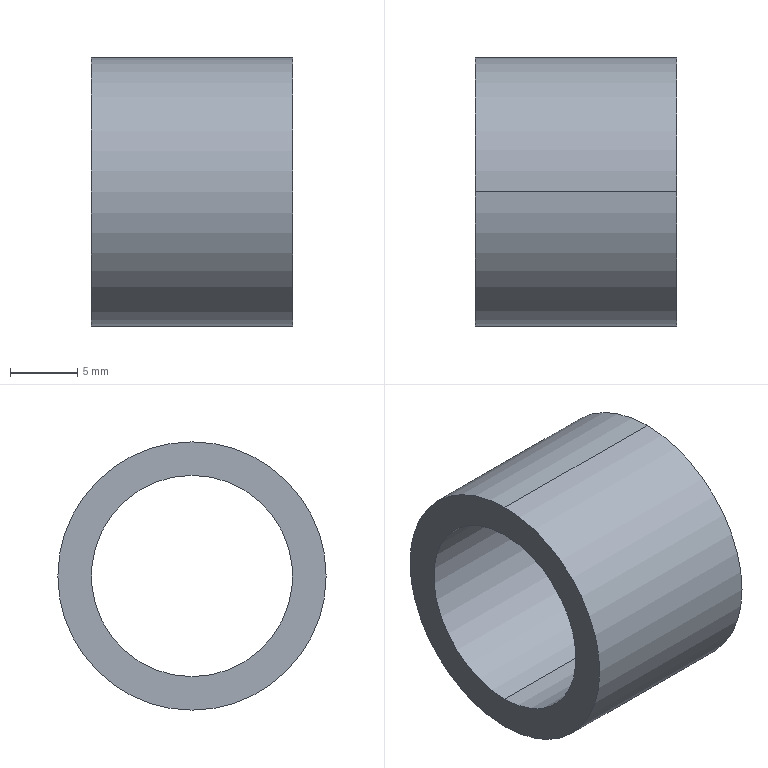Part | NX | features BREP 1 | 1 solid | 6 faces | box 15 x 20 x 20 mm | volume 2062 mm3 | cylinder 4 | plane 2 | commonest cylinder face diameters 15 x2 20 x2
STEP:
#1=CARTESIAN_POINT('',(15.,0.,10.));
#2=VERTEX_POINT('',#1);
#3=CARTESIAN_POINT('',(15.,0.,-10.));
#4=VERTEX_POINT('',#3);
#5=CARTESIAN_POINT('',(15.,0.,0.));
#6=DIRECTION('',(1.,0.,0.));
#7=DIRECTION('',(0.,0.,1.));
#8=AXIS2_PLACEMENT_3D('',#5,#6,#7);
#9=CIRCLE('',#8,10.);
#10=EDGE_CURVE('',#2,#4,#9,.T.);
#11=ORIENTED_EDGE('',*,*,#10,.T.);
#12=CARTESIAN_POINT('',(15.,0.,0.));
#13=DIRECTION('',(1.,0.,0.));
#14=DIRECTION('',(0.,0.,-1.));
#15=AXIS2_PLACEMENT_3D('',#12,#13,#14);
#16=CIRCLE('',#15,10.);
#17=EDGE_CURVE('',#4,#2,#16,.T.);
#18=ORIENTED_EDGE('',*,*,#17,.T.);
#19=EDGE_LOOP('',(#11,#18));
#20=FACE_BOUND('',#19,.T.);
#21=CARTESIAN_POINT('',(15.,0.,7.5));
#22=VERTEX_POINT('',#21);
#23=CARTESIAN_POINT('',(15.,0.,-7.5));
#24=VERTEX_POINT('',#23);
#25=CARTESIAN_POINT('',(15.,0.,0.));
#26=DIRECTION('',(-1.,0.,0.));
#27=DIRECTION('',(0.,0.,1.));
#28=AXIS2_PLACEMENT_3D('',#25,#26,#27);
#29=CIRCLE('',#28,7.5);
#30=EDGE_CURVE('',#22,#24,#29,.T.);
#31=ORIENTED_EDGE('',*,*,#30,.T.);
#32=CARTESIAN_POINT('',(15.,0.,0.));
#33=DIRECTION('',(-1.,0.,0.));
#34=DIRECTION('',(0.,0.,-1.));
#35=AXIS2_PLACEMENT_3D('',#32,#33,#34);
#36=CIRCLE('',#35,7.5);
#37=EDGE_CURVE('',#24,#22,#36,.T.);
#38=ORIENTED_EDGE('',*,*,#37,.T.);
#39=EDGE_LOOP('',(#31,#38));
#40=FACE_BOUND('',#39,.T.);
#41=CARTESIAN_POINT('',(15.,7.5,0.));
#42=DIRECTION('',(1.,0.,0.));
#43=DIRECTION('',(0.,1.,0.));
#44=AXIS2_PLACEMENT_3D('',#41,#42,#43);
#45=PLANE('',#44);
#46=ADVANCED_FACE('',(#20,#40),#45,.T.);
#47=CARTESIAN_POINT('',(0.,0.,-10.));
#48=VERTEX_POINT('',#47);
#49=CARTESIAN_POINT('',(15.,0.,-10.));
#50=DIRECTION('',(-1.,0.,0.));
#51=VECTOR('',#50,1000.);
#52=LINE('',#49,#51);
#53=EDGE_CURVE('',#4,#48,#52,.T.);
#54=ORIENTED_EDGE('',*,*,#53,.T.);
#55=CARTESIAN_POINT('',(0.,0.,10.));
#56=VERTEX_POINT('',#55);
#57=CARTESIAN_POINT('',(0.,0.,0.));
#58=DIRECTION('',(-1.,0.,0.));
#59=DIRECTION('',(0.,0.,1.));
#60=AXIS2_PLACEMENT_3D('',#57,#58,#59);
#61=CIRCLE('',#60,10.);
#62=EDGE_CURVE('',#56,#48,#61,.T.);
#63=ORIENTED_EDGE('',*,*,#62,.F.);
#64=CARTESIAN_POINT('',(15.,0.,10.));
#65=DIRECTION('',(-1.,0.,0.));
#66=VECTOR('',#65,1000.);
#67=LINE('',#64,#66);
#68=EDGE_CURVE('',#2,#56,#67,.T.);
#69=ORIENTED_EDGE('',*,*,#68,.F.);
#70=ORIENTED_EDGE('',*,*,#17,.F.);
#71=EDGE_LOOP('',(#54,#63,#69,#70));
#72=FACE_BOUND('',#71,.T.);
#73=CARTESIAN_POINT('',(15.,0.,0.));
#74=DIRECTION('',(-1.,0.,0.));
#75=DIRECTION('',(0.,0.,-1.));
#76=AXIS2_PLACEMENT_3D('',#73,#74,#75);
#77=CYLINDRICAL_SURFACE('',#76,10.);
#78=ADVANCED_FACE('',(#72),#77,.T.);
#79=ORIENTED_EDGE('',*,*,#68,.T.);
#80=CARTESIAN_POINT('',(0.,0.,0.));
#81=DIRECTION('',(-1.,0.,0.));
#82=DIRECTION('',(0.,0.,-1.));
#83=AXIS2_PLACEMENT_3D('',#80,#81,#82);
#84=CIRCLE('',#83,10.);
#85=EDGE_CURVE('',#48,#56,#84,.T.);
#86=ORIENTED_EDGE('',*,*,#85,.F.);
#87=ORIENTED_EDGE('',*,*,#53,.F.);
#88=ORIENTED_EDGE('',*,*,#10,.F.);
#89=EDGE_LOOP('',(#79,#86,#87,#88));
#90=FACE_BOUND('',#89,.T.);
#91=CARTESIAN_POINT('',(15.,0.,0.));
#92=DIRECTION('',(-1.,0.,0.));
#93=DIRECTION('',(0.,0.,-1.));
#94=AXIS2_PLACEMENT_3D('',#91,#92,#93);
#95=CYLINDRICAL_SURFACE('',#94,10.);
#96=ADVANCED_FACE('',(#90),#95,.T.);
#97=ORIENTED_EDGE('',*,*,#62,.T.);
#98=ORIENTED_EDGE('',*,*,#85,.T.);
#99=EDGE_LOOP('',(#97,#98));
#100=FACE_BOUND('',#99,.T.);
#101=CARTESIAN_POINT('',(0.,0.,7.5));
#102=VERTEX_POINT('',#101);
#103=CARTESIAN_POINT('',(0.,0.,-7.5));
#104=VERTEX_POINT('',#103);
#105=CARTESIAN_POINT('',(0.,0.,0.));
#106=DIRECTION('',(1.,0.,0.));
#107=DIRECTION('',(0.,0.,1.));
#108=AXIS2_PLACEMENT_3D('',#105,#106,#107);
#109=CIRCLE('',#108,7.5);
#110=EDGE_CURVE('',#102,#104,#109,.T.);
#111=ORIENTED_EDGE('',*,*,#110,.T.);
#112=CARTESIAN_POINT('',(0.,0.,0.));
#113=DIRECTION('',(1.,0.,0.));
#114=DIRECTION('',(0.,0.,-1.));
#115=AXIS2_PLACEMENT_3D('',#112,#113,#114);
#116=CIRCLE('',#115,7.5);
#117=EDGE_CURVE('',#104,#102,#116,.T.);
#118=ORIENTED_EDGE('',*,*,#117,.T.);
#119=EDGE_LOOP('',(#111,#118));
#120=FACE_BOUND('',#119,.T.);
#121=CARTESIAN_POINT('',(0.,10.,0.));
#122=DIRECTION('',(-1.,0.,0.));
#123=DIRECTION('',(0.,0.,1.));
#124=AXIS2_PLACEMENT_3D('',#121,#122,#123);
#125=PLANE('',#124);
#126=ADVANCED_FACE('',(#100,#120),#125,.T.);
#127=CARTESIAN_POINT('',(15.,0.,-7.5));
#128=DIRECTION('',(-1.,0.,0.));
#129=VECTOR('',#128,1000.);
#130=LINE('',#127,#129);
#131=EDGE_CURVE('',#24,#104,#130,.T.);
#132=ORIENTED_EDGE('',*,*,#131,.F.);
#133=ORIENTED_EDGE('',*,*,#30,.F.);
#134=CARTESIAN_POINT('',(15.,0.,7.5));
#135=DIRECTION('',(-1.,0.,0.));
#136=VECTOR('',#135,1000.);
#137=LINE('',#134,#136);
#138=EDGE_CURVE('',#22,#102,#137,.T.);
#139=ORIENTED_EDGE('',*,*,#138,.T.);
#140=ORIENTED_EDGE('',*,*,#117,.F.);
#141=EDGE_LOOP('',(#132,#133,#139,#140));
#142=FACE_BOUND('',#141,.T.);
#143=CARTESIAN_POINT('',(15.,0.,0.));
#144=DIRECTION('',(-1.,0.,0.));
#145=DIRECTION('',(0.,0.,-1.));
#146=AXIS2_PLACEMENT_3D('',#143,#144,#145);
#147=CYLINDRICAL_SURFACE('',#146,7.5);
#148=ADVANCED_FACE('',(#142),#147,.F.);
#149=ORIENTED_EDGE('',*,*,#138,.F.);
#150=ORIENTED_EDGE('',*,*,#37,.F.);
#151=ORIENTED_EDGE('',*,*,#131,.T.);
#152=ORIENTED_EDGE('',*,*,#110,.F.);
#153=EDGE_LOOP('',(#149,#150,#151,#152));
#154=FACE_BOUND('',#153,.T.);
#155=CARTESIAN_POINT('',(15.,0.,0.));
#156=DIRECTION('',(-1.,0.,0.));
#157=DIRECTION('',(0.,0.,-1.));
#158=AXIS2_PLACEMENT_3D('',#155,#156,#157);
#159=CYLINDRICAL_SURFACE('',#158,7.5);
#160=ADVANCED_FACE('',(#154),#159,.F.);
#161=CLOSED_SHELL('',(#46,#78,#96,#126,#148,#160));
#162=MANIFOLD_SOLID_BREP('',#161);
#163=(LENGTH_UNIT()NAMED_UNIT(*)SI_UNIT(.MILLI.,.METRE.));
#164=UNCERTAINTY_MEASURE_WITH_UNIT(LENGTH_MEASURE(0.00001),#163,'','');
#165=(NAMED_UNIT(*)PLANE_ANGLE_UNIT()SI_UNIT($,.RADIAN.));
#166=(NAMED_UNIT(*)SI_UNIT($,.STERADIAN.)SOLID_ANGLE_UNIT());
#167=(GEOMETRIC_REPRESENTATION_CONTEXT(3)GLOBAL_UNCERTAINTY_ASSIGNED_CONTEXT((#164))GLOBAL_UNIT_ASSIGNED_CONTEXT((#163,#165,#166))REPRESENTATION_CONTEXT('',''));
#168=ADVANCED_BREP_SHAPE_REPRESENTATION('',(#162),#167);